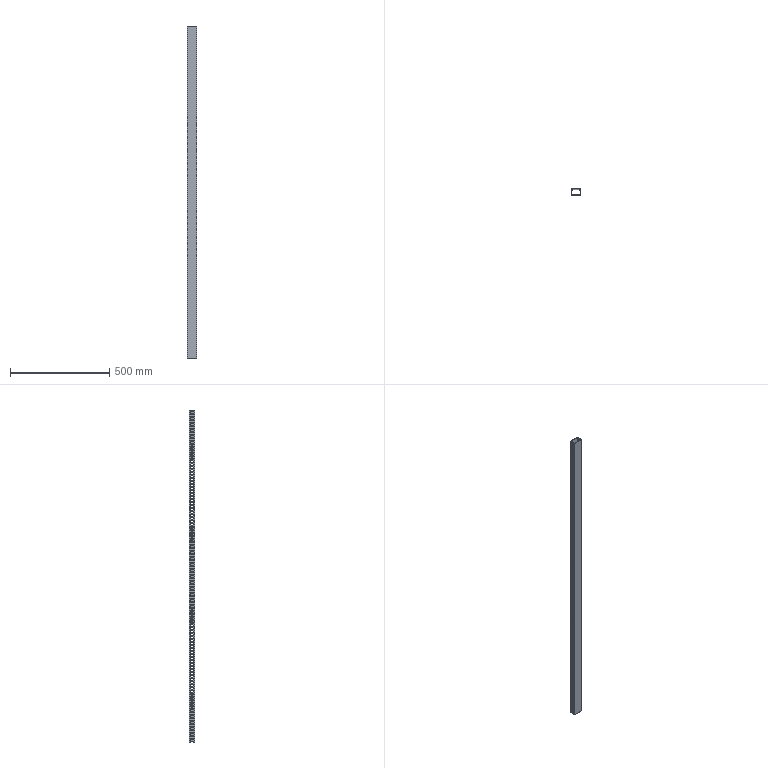Part | SolidWorks | features BaseBody 1 | 1 solid | 921 faces | box 50 x 30 x 1670 mm | volume 272007 mm3 | plane 473 | cylinder 448 | commonest cylinder face diameters 8 x448